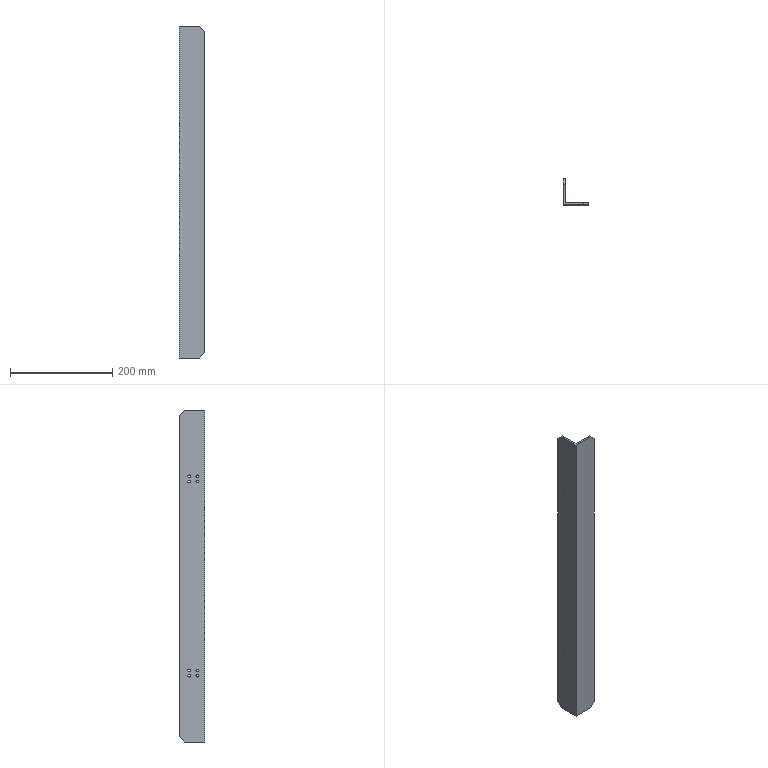Part | SolidWorks | features Chamfer 1, Extrusion 1, HoleWzd 1 | 1 solid | 44 faces | box 50 x 50 x 650 mm | volume 247288 mm3 | cylinder 16 | cone 16 | plane 12 | commonest cylinder face diameters 5.5 x16
STEP:
#1=CARTESIAN_POINT('',(0.,30.5,197.75));
#2=VERTEX_POINT('',#1);
#3=CARTESIAN_POINT('',(0.,30.5,192.25));
#4=VERTEX_POINT('',#3);
#5=CARTESIAN_POINT('',(0.,30.5,195.));
#6=DIRECTION('',(1.,0.,0.));
#7=DIRECTION('',(0.,0.,-1.));
#8=AXIS2_PLACEMENT_3D('',#5,#6,#7);
#9=CIRCLE('',#8,2.75);
#10=EDGE_CURVE('',#2,#4,#9,.T.);
#11=ORIENTED_EDGE('',*,*,#10,.F.);
#12=CARTESIAN_POINT('',(1.15,30.5,197.75));
#13=VERTEX_POINT('',#12);
#14=CARTESIAN_POINT('',(4.,30.5,197.75));
#15=DIRECTION('',(1.,0.,0.));
#16=VECTOR('',#15,1000.);
#17=LINE('',#14,#16);
#18=EDGE_CURVE('',#2,#13,#17,.T.);
#19=ORIENTED_EDGE('',*,*,#18,.T.);
#20=CARTESIAN_POINT('',(1.15,30.5,192.25));
#21=VERTEX_POINT('',#20);
#22=CARTESIAN_POINT('',(1.15,30.5,195.));
#23=DIRECTION('',(1.,0.,0.));
#24=DIRECTION('',(0.,0.,-1.));
#25=AXIS2_PLACEMENT_3D('',#22,#23,#24);
#26=CIRCLE('',#25,2.75);
#27=EDGE_CURVE('',#13,#21,#26,.T.);
#28=ORIENTED_EDGE('',*,*,#27,.T.);
#29=CARTESIAN_POINT('',(4.,30.5,192.25));
#30=DIRECTION('',(1.,0.,0.));
#31=VECTOR('',#30,1000.);
#32=LINE('',#29,#31);
#33=EDGE_CURVE('',#4,#21,#32,.T.);
#34=ORIENTED_EDGE('',*,*,#33,.F.);
#35=EDGE_LOOP('',(#11,#19,#28,#34));
#36=FACE_OUTER_BOUND('',#35,.T.);
#37=CARTESIAN_POINT('',(4.,30.5,195.));
#38=DIRECTION('',(1.,0.,0.));
#39=DIRECTION('',(0.,0.,-1.));
#40=AXIS2_PLACEMENT_3D('',#37,#38,#39);
#41=CYLINDRICAL_SURFACE('',#40,2.75);
#42=ADVANCED_FACE('',(#36),#41,.F.);
#43=ORIENTED_EDGE('',*,*,#27,.F.);
#44=CARTESIAN_POINT('',(4.,30.5,200.6));
#45=VERTEX_POINT('',#44);
#46=CARTESIAN_POINT('',(4.,30.5,200.6));
#47=DIRECTION('',(0.7071,0.,0.7071));
#48=VECTOR('',#47,1000.);
#49=LINE('',#46,#48);
#50=EDGE_CURVE('',#13,#45,#49,.T.);
#51=ORIENTED_EDGE('',*,*,#50,.T.);
#52=CARTESIAN_POINT('',(4.,27.978,190.));
#53=VERTEX_POINT('',#52);
#54=CARTESIAN_POINT('',(4.,30.5,195.));
#55=DIRECTION('',(1.,0.,0.));
#56=DIRECTION('',(0.,0.,-1.));
#57=AXIS2_PLACEMENT_3D('',#54,#55,#56);
#58=CIRCLE('',#57,5.6);
#59=EDGE_CURVE('',#45,#53,#58,.T.);
#60=ORIENTED_EDGE('',*,*,#59,.T.);
#61=CARTESIAN_POINT('',(3.4,30.5,190.));
#62=VERTEX_POINT('',#61);
#63=CARTESIAN_POINT('',(3.4,30.5,190.));
#64=CARTESIAN_POINT('',(3.4,30.063,190.));
#65=CARTESIAN_POINT('',(3.458,29.635,190.));
#66=CARTESIAN_POINT('',(3.668,28.793,190.));
#67=CARTESIAN_POINT('',(3.82,28.378,190.));
#68=CARTESIAN_POINT('',(4.,27.978,190.));
#69=B_SPLINE_CURVE_WITH_KNOTS('',3,(#63,#64,#65,#66,#67,#68),.UNSPECIFIED.,.F.,.F.,(4,2,4),(0.002595,0.003891,0.005187),.UNSPECIFIED.);
#70=EDGE_CURVE('',#62,#53,#69,.T.);
#71=ORIENTED_EDGE('',*,*,#70,.F.);
#72=CARTESIAN_POINT('',(4.,30.5,189.4));
#73=DIRECTION('',(0.7071,0.,-0.7071));
#74=VECTOR('',#73,1000.);
#75=LINE('',#72,#74);
#76=EDGE_CURVE('',#21,#62,#75,.T.);
#77=ORIENTED_EDGE('',*,*,#76,.F.);
#78=EDGE_LOOP('',(#43,#51,#60,#71,#77));
#79=FACE_OUTER_BOUND('',#78,.T.);
#80=CARTESIAN_POINT('',(4.,30.5,195.));
#81=DIRECTION('',(1.,0.,0.));
#82=DIRECTION('',(0.,0.,-1.));
#83=AXIS2_PLACEMENT_3D('',#80,#81,#82);
#84=CONICAL_SURFACE('',#83,5.6,0.7854);
#85=ADVANCED_FACE('',(#79),#84,.F.);
#86=CARTESIAN_POINT('',(0.,30.5,-182.25));
#87=VERTEX_POINT('',#86);
#88=CARTESIAN_POINT('',(0.,30.5,-187.75));
#89=VERTEX_POINT('',#88);
#90=CARTESIAN_POINT('',(0.,30.5,-185.));
#91=DIRECTION('',(1.,0.,0.));
#92=DIRECTION('',(0.,0.,-1.));
#93=AXIS2_PLACEMENT_3D('',#90,#91,#92);
#94=CIRCLE('',#93,2.75);
#95=EDGE_CURVE('',#87,#89,#94,.T.);
#96=ORIENTED_EDGE('',*,*,#95,.F.);
#97=CARTESIAN_POINT('',(1.15,30.5,-182.25));
#98=VERTEX_POINT('',#97);
#99=CARTESIAN_POINT('',(4.,30.5,-182.25));
#100=DIRECTION('',(1.,0.,0.));
#101=VECTOR('',#100,1000.);
#102=LINE('',#99,#101);
#103=EDGE_CURVE('',#87,#98,#102,.T.);
#104=ORIENTED_EDGE('',*,*,#103,.T.);
#105=CARTESIAN_POINT('',(1.15,30.5,-187.75));
#106=VERTEX_POINT('',#105);
#107=CARTESIAN_POINT('',(1.15,30.5,-185.));
#108=DIRECTION('',(1.,0.,0.));
#109=DIRECTION('',(0.,0.,-1.));
#110=AXIS2_PLACEMENT_3D('',#107,#108,#109);
#111=CIRCLE('',#110,2.75);
#112=EDGE_CURVE('',#98,#106,#111,.T.);
#113=ORIENTED_EDGE('',*,*,#112,.T.);
#114=CARTESIAN_POINT('',(4.,30.5,-187.75));
#115=DIRECTION('',(1.,0.,0.));
#116=VECTOR('',#115,1000.);
#117=LINE('',#114,#116);
#118=EDGE_CURVE('',#89,#106,#117,.T.);
#119=ORIENTED_EDGE('',*,*,#118,.F.);
#120=EDGE_LOOP('',(#96,#104,#113,#119));
#121=FACE_OUTER_BOUND('',#120,.T.);
#122=CARTESIAN_POINT('',(4.,30.5,-185.));
#123=DIRECTION('',(1.,0.,0.));
#124=DIRECTION('',(0.,0.,-1.));
#125=AXIS2_PLACEMENT_3D('',#122,#123,#124);
#126=CYLINDRICAL_SURFACE('',#125,2.75);
#127=ADVANCED_FACE('',(#121),#126,.F.);
#128=ORIENTED_EDGE('',*,*,#112,.F.);
#129=CARTESIAN_POINT('',(4.,30.5,-179.4));
#130=VERTEX_POINT('',#129);
#131=CARTESIAN_POINT('',(4.,30.5,-179.4));
#132=DIRECTION('',(0.7071,0.,0.7071));
#133=VECTOR('',#132,1000.);
#134=LINE('',#131,#133);
#135=EDGE_CURVE('',#98,#130,#134,.T.);
#136=ORIENTED_EDGE('',*,*,#135,.T.);
#137=CARTESIAN_POINT('',(4.,27.978,-190.));
#138=VERTEX_POINT('',#137);
#139=CARTESIAN_POINT('',(4.,30.5,-185.));
#140=DIRECTION('',(1.,0.,0.));
#141=DIRECTION('',(0.,0.,-1.));
#142=AXIS2_PLACEMENT_3D('',#139,#140,#141);
#143=CIRCLE('',#142,5.6);
#144=EDGE_CURVE('',#130,#138,#143,.T.);
#145=ORIENTED_EDGE('',*,*,#144,.T.);
#146=CARTESIAN_POINT('',(3.4,30.5,-190.));
#147=VERTEX_POINT('',#146);
#148=CARTESIAN_POINT('',(3.4,30.5,-190.));
#149=CARTESIAN_POINT('',(3.4,30.063,-190.));
#150=CARTESIAN_POINT('',(3.458,29.635,-190.));
#151=CARTESIAN_POINT('',(3.668,28.793,-190.));
#152=CARTESIAN_POINT('',(3.82,28.378,-190.));
#153=CARTESIAN_POINT('',(4.,27.978,-190.));
#154=B_SPLINE_CURVE_WITH_KNOTS('',3,(#148,#149,#150,#151,#152,#153),.UNSPECIFIED.,.F.,.F.,(4,2,4),(0.002595,0.003891,0.005187),.UNSPECIFIED.);
#155=EDGE_CURVE('',#147,#138,#154,.T.);
#156=ORIENTED_EDGE('',*,*,#155,.F.);
#157=CARTESIAN_POINT('',(4.,30.5,-190.6));
#158=DIRECTION('',(0.7071,0.,-0.7071));
#159=VECTOR('',#158,1000.);
#160=LINE('',#157,#159);
#161=EDGE_CURVE('',#106,#147,#160,.T.);
#162=ORIENTED_EDGE('',*,*,#161,.F.);
#163=EDGE_LOOP('',(#128,#136,#145,#156,#162));
#164=FACE_OUTER_BOUND('',#163,.T.);
#165=CARTESIAN_POINT('',(4.,30.5,-185.));
#166=DIRECTION('',(1.,0.,0.));
#167=DIRECTION('',(0.,0.,-1.));
#168=AXIS2_PLACEMENT_3D('',#165,#166,#167);
#169=CONICAL_SURFACE('',#168,5.6,0.7854);
#170=ADVANCED_FACE('',(#164),#169,.F.);
#171=CARTESIAN_POINT('',(1.15,30.5,187.75));
#172=VERTEX_POINT('',#171);
#173=CARTESIAN_POINT('',(1.15,30.5,182.25));
#174=VERTEX_POINT('',#173);
#175=CARTESIAN_POINT('',(1.15,30.5,185.));
#176=DIRECTION('',(1.,0.,0.));
#177=DIRECTION('',(0.,0.,-1.));
#178=AXIS2_PLACEMENT_3D('',#175,#176,#177);
#179=CIRCLE('',#178,2.75);
#180=EDGE_CURVE('',#172,#174,#179,.T.);
#181=ORIENTED_EDGE('',*,*,#180,.F.);
#182=CARTESIAN_POINT('',(4.,30.5,190.6));
#183=DIRECTION('',(0.7071,0.,0.7071));
#184=VECTOR('',#183,1000.);
#185=LINE('',#182,#184);
#186=EDGE_CURVE('',#172,#62,#185,.T.);
#187=ORIENTED_EDGE('',*,*,#186,.T.);
#188=ORIENTED_EDGE('',*,*,#70,.T.);
#189=CARTESIAN_POINT('',(4.,30.5,179.4));
#190=VERTEX_POINT('',#189);
#191=CARTESIAN_POINT('',(4.,30.5,185.));
#192=DIRECTION('',(1.,0.,0.));
#193=DIRECTION('',(0.,0.,-1.));
#194=AXIS2_PLACEMENT_3D('',#191,#192,#193);
#195=CIRCLE('',#194,5.6);
#196=EDGE_CURVE('',#53,#190,#195,.T.);
#197=ORIENTED_EDGE('',*,*,#196,.T.);
#198=CARTESIAN_POINT('',(4.,30.5,179.4));
#199=DIRECTION('',(0.7071,0.,-0.7071));
#200=VECTOR('',#199,1000.);
#201=LINE('',#198,#200);
#202=EDGE_CURVE('',#174,#190,#201,.T.);
#203=ORIENTED_EDGE('',*,*,#202,.F.);
#204=EDGE_LOOP('',(#181,#187,#188,#197,#203));
#205=FACE_OUTER_BOUND('',#204,.T.);
#206=CARTESIAN_POINT('',(4.,30.5,185.));
#207=DIRECTION('',(1.,0.,0.));
#208=DIRECTION('',(0.,0.,-1.));
#209=AXIS2_PLACEMENT_3D('',#206,#207,#208);
#210=CONICAL_SURFACE('',#209,5.6,0.7854);
#211=ADVANCED_FACE('',(#205),#210,.F.);
#212=CARTESIAN_POINT('',(0.,30.5,187.75));
#213=VERTEX_POINT('',#212);
#214=CARTESIAN_POINT('',(0.,30.5,182.25));
#215=VERTEX_POINT('',#214);
#216=CARTESIAN_POINT('',(0.,30.5,185.));
#217=DIRECTION('',(1.,0.,0.));
#218=DIRECTION('',(0.,0.,-1.));
#219=AXIS2_PLACEMENT_3D('',#216,#217,#218);
#220=CIRCLE('',#219,2.75);
#221=EDGE_CURVE('',#213,#215,#220,.T.);
#222=ORIENTED_EDGE('',*,*,#221,.F.);
#223=CARTESIAN_POINT('',(4.,30.5,187.75));
#224=DIRECTION('',(1.,0.,0.));
#225=VECTOR('',#224,1000.);
#226=LINE('',#223,#225);
#227=EDGE_CURVE('',#213,#172,#226,.T.);
#228=ORIENTED_EDGE('',*,*,#227,.T.);
#229=ORIENTED_EDGE('',*,*,#180,.T.);
#230=CARTESIAN_POINT('',(4.,30.5,182.25));
#231=DIRECTION('',(1.,0.,0.));
#232=VECTOR('',#231,1000.);
#233=LINE('',#230,#232);
#234=EDGE_CURVE('',#215,#174,#233,.T.);
#235=ORIENTED_EDGE('',*,*,#234,.F.);
#236=EDGE_LOOP('',(#222,#228,#229,#235));
#237=FACE_OUTER_BOUND('',#236,.T.);
#238=CARTESIAN_POINT('',(4.,30.5,185.));
#239=DIRECTION('',(1.,0.,0.));
#240=DIRECTION('',(0.,0.,-1.));
#241=AXIS2_PLACEMENT_3D('',#238,#239,#240);
#242=CYLINDRICAL_SURFACE('',#241,2.75);
#243=ADVANCED_FACE('',(#237),#242,.F.);
#244=CARTESIAN_POINT('',(1.15,30.5,-192.25));
#245=VERTEX_POINT('',#244);
#246=CARTESIAN_POINT('',(1.15,30.5,-197.75));
#247=VERTEX_POINT('',#246);
#248=CARTESIAN_POINT('',(1.15,30.5,-195.));
#249=DIRECTION('',(1.,0.,0.));
#250=DIRECTION('',(0.,0.,-1.));
#251=AXIS2_PLACEMENT_3D('',#248,#249,#250);
#252=CIRCLE('',#251,2.75);
#253=EDGE_CURVE('',#245,#247,#252,.T.);
#254=ORIENTED_EDGE('',*,*,#253,.F.);
#255=CARTESIAN_POINT('',(4.,30.5,-189.4));
#256=DIRECTION('',(0.7071,0.,0.7071));
#257=VECTOR('',#256,1000.);
#258=LINE('',#255,#257);
#259=EDGE_CURVE('',#245,#147,#258,.T.);
#260=ORIENTED_EDGE('',*,*,#259,.T.);
#261=ORIENTED_EDGE('',*,*,#155,.T.);
#262=CARTESIAN_POINT('',(4.,30.5,-200.6));
#263=VERTEX_POINT('',#262);
#264=CARTESIAN_POINT('',(4.,30.5,-195.));
#265=DIRECTION('',(1.,0.,0.));
#266=DIRECTION('',(0.,0.,-1.));
#267=AXIS2_PLACEMENT_3D('',#264,#265,#266);
#268=CIRCLE('',#267,5.6);
#269=EDGE_CURVE('',#138,#263,#268,.T.);
#270=ORIENTED_EDGE('',*,*,#269,.T.);
#271=CARTESIAN_POINT('',(4.,30.5,-200.6));
#272=DIRECTION('',(0.7071,0.,-0.7071));
#273=VECTOR('',#272,1000.);
#274=LINE('',#271,#273);
#275=EDGE_CURVE('',#247,#263,#274,.T.);
#276=ORIENTED_EDGE('',*,*,#275,.F.);
#277=EDGE_LOOP('',(#254,#260,#261,#270,#276));
#278=FACE_OUTER_BOUND('',#277,.T.);
#279=CARTESIAN_POINT('',(4.,30.5,-195.));
#280=DIRECTION('',(1.,0.,0.));
#281=DIRECTION('',(0.,0.,-1.));
#282=AXIS2_PLACEMENT_3D('',#279,#280,#281);
#283=CONICAL_SURFACE('',#282,5.6,0.7854);
#284=ADVANCED_FACE('',(#278),#283,.F.);
#285=CARTESIAN_POINT('',(0.,30.5,-192.25));
#286=VERTEX_POINT('',#285);
#287=CARTESIAN_POINT('',(0.,30.5,-197.75));
#288=VERTEX_POINT('',#287);
#289=CARTESIAN_POINT('',(0.,30.5,-195.));
#290=DIRECTION('',(1.,0.,0.));
#291=DIRECTION('',(0.,0.,-1.));
#292=AXIS2_PLACEMENT_3D('',#289,#290,#291);
#293=CIRCLE('',#292,2.75);
#294=EDGE_CURVE('',#286,#288,#293,.T.);
#295=ORIENTED_EDGE('',*,*,#294,.F.);
#296=CARTESIAN_POINT('',(4.,30.5,-192.25));
#297=DIRECTION('',(1.,0.,0.));
#298=VECTOR('',#297,1000.);
#299=LINE('',#296,#298);
#300=EDGE_CURVE('',#286,#245,#299,.T.);
#301=ORIENTED_EDGE('',*,*,#300,.T.);
#302=ORIENTED_EDGE('',*,*,#253,.T.);
#303=CARTESIAN_POINT('',(4.,30.5,-197.75));
#304=DIRECTION('',(1.,0.,0.));
#305=VECTOR('',#304,1000.);
#306=LINE('',#303,#305);
#307=EDGE_CURVE('',#288,#247,#306,.T.);
#308=ORIENTED_EDGE('',*,*,#307,.F.);
#309=EDGE_LOOP('',(#295,#301,#302,#308));
#310=FACE_OUTER_BOUND('',#309,.T.);
#311=CARTESIAN_POINT('',(4.,30.5,-195.));
#312=DIRECTION('',(1.,0.,0.));
#313=DIRECTION('',(0.,0.,-1.));
#314=AXIS2_PLACEMENT_3D('',#311,#312,#313);
#315=CYLINDRICAL_SURFACE('',#314,2.75);
#316=ADVANCED_FACE('',(#310),#315,.F.);
#317=CARTESIAN_POINT('',(0.,14.5,197.75));
#318=VERTEX_POINT('',#317);
#319=CARTESIAN_POINT('',(0.,14.5,192.25));
#320=VERTEX_POINT('',#319);
#321=CARTESIAN_POINT('',(0.,14.5,195.));
#322=DIRECTION('',(1.,0.,0.));
#323=DIRECTION('',(0.,0.,-1.));
#324=AXIS2_PLACEMENT_3D('',#321,#322,#323);
#325=CIRCLE('',#324,2.75);
#326=EDGE_CURVE('',#318,#320,#325,.T.);
#327=ORIENTED_EDGE('',*,*,#326,.F.);
#328=CARTESIAN_POINT('',(1.15,14.5,197.75));
#329=VERTEX_POINT('',#328);
#330=CARTESIAN_POINT('',(4.,14.5,197.75));
#331=DIRECTION('',(1.,0.,0.));
#332=VECTOR('',#331,1000.);
#333=LINE('',#330,#332);
#334=EDGE_CURVE('',#318,#329,#333,.T.);
#335=ORIENTED_EDGE('',*,*,#334,.T.);
#336=CARTESIAN_POINT('',(1.15,14.5,192.25));
#337=VERTEX_POINT('',#336);
#338=CARTESIAN_POINT('',(1.15,14.5,195.));
#339=DIRECTION('',(1.,0.,0.));
#340=DIRECTION('',(0.,0.,-1.));
#341=AXIS2_PLACEMENT_3D('',#338,#339,#340);
#342=CIRCLE('',#341,2.75);
#343=EDGE_CURVE('',#329,#337,#342,.T.);
#344=ORIENTED_EDGE('',*,*,#343,.T.);
#345=CARTESIAN_POINT('',(4.,14.5,192.25));
#346=DIRECTION('',(1.,0.,0.));
#347=VECTOR('',#346,1000.);
#348=LINE('',#345,#347);
#349=EDGE_CURVE('',#320,#337,#348,.T.);
#350=ORIENTED_EDGE('',*,*,#349,.F.);
#351=EDGE_LOOP('',(#327,#335,#344,#350));
#352=FACE_OUTER_BOUND('',#351,.T.);
#353=CARTESIAN_POINT('',(4.,14.5,195.));
#354=DIRECTION('',(1.,0.,0.));
#355=DIRECTION('',(0.,0.,-1.));
#356=AXIS2_PLACEMENT_3D('',#353,#354,#355);
#357=CYLINDRICAL_SURFACE('',#356,2.75);
#358=ADVANCED_FACE('',(#352),#357,.F.);
#359=ORIENTED_EDGE('',*,*,#343,.F.);
#360=CARTESIAN_POINT('',(4.,14.5,200.6));
#361=VERTEX_POINT('',#360);
#362=CARTESIAN_POINT('',(4.,14.5,200.6));
#363=DIRECTION('',(0.7071,0.,0.7071));
#364=VECTOR('',#363,1000.);
#365=LINE('',#362,#364);
#366=EDGE_CURVE('',#329,#361,#365,.T.);
#367=ORIENTED_EDGE('',*,*,#366,.T.);
#368=CARTESIAN_POINT('',(4.,11.978,190.));
#369=VERTEX_POINT('',#368);
#370=CARTESIAN_POINT('',(4.,14.5,195.));
#371=DIRECTION('',(1.,0.,0.));
#372=DIRECTION('',(0.,0.,-1.));
#373=AXIS2_PLACEMENT_3D('',#370,#371,#372);
#374=CIRCLE('',#373,5.6);
#375=EDGE_CURVE('',#361,#369,#374,.T.);
#376=ORIENTED_EDGE('',*,*,#375,.T.);
#377=CARTESIAN_POINT('',(3.4,14.5,190.));
#378=VERTEX_POINT('',#377);
#379=CARTESIAN_POINT('',(3.4,14.5,190.));
#380=CARTESIAN_POINT('',(3.4,14.063,190.));
#381=CARTESIAN_POINT('',(3.458,13.635,190.));
#382=CARTESIAN_POINT('',(3.668,12.793,190.));
#383=CARTESIAN_POINT('',(3.82,12.378,190.));
#384=CARTESIAN_POINT('',(4.,11.978,190.));
#385=B_SPLINE_CURVE_WITH_KNOTS('',3,(#379,#380,#381,#382,#383,#384),.UNSPECIFIED.,.F.,.F.,(4,2,4),(0.002595,0.003891,0.005187),.UNSPECIFIED.);
#386=EDGE_CURVE('',#378,#369,#385,.T.);
#387=ORIENTED_EDGE('',*,*,#386,.F.);
#388=CARTESIAN_POINT('',(4.,14.5,189.4));
#389=DIRECTION('',(0.7071,0.,-0.7071));
#390=VECTOR('',#389,1000.);
#391=LINE('',#388,#390);
#392=EDGE_CURVE('',#337,#378,#391,.T.);
#393=ORIENTED_EDGE('',*,*,#392,.F.);
#394=EDGE_LOOP('',(#359,#367,#376,#387,#393));
#395=FACE_OUTER_BOUND('',#394,.T.);
#396=CARTESIAN_POINT('',(4.,14.5,195.));
#397=DIRECTION('',(1.,0.,0.));
#398=DIRECTION('',(0.,0.,-1.));
#399=AXIS2_PLACEMENT_3D('',#396,#397,#398);
#400=CONICAL_SURFACE('',#399,5.6,0.7854);
#401=ADVANCED_FACE('',(#395),#400,.F.);
#402=CARTESIAN_POINT('',(0.,14.5,-182.25));
#403=VERTEX_POINT('',#402);
#404=CARTESIAN_POINT('',(0.,14.5,-187.75));
#405=VERTEX_POINT('',#404);
#406=CARTESIAN_POINT('',(0.,14.5,-185.));
#407=DIRECTION('',(1.,0.,0.));
#408=DIRECTION('',(0.,0.,-1.));
#409=AXIS2_PLACEMENT_3D('',#406,#407,#408);
#410=CIRCLE('',#409,2.75);
#411=EDGE_CURVE('',#403,#405,#410,.T.);
#412=ORIENTED_EDGE('',*,*,#411,.F.);
#413=CARTESIAN_POINT('',(1.15,14.5,-182.25));
#414=VERTEX_POINT('',#413);
#415=CARTESIAN_POINT('',(4.,14.5,-182.25));
#416=DIRECTION('',(1.,0.,0.));
#417=VECTOR('',#416,1000.);
#418=LINE('',#415,#417);
#419=EDGE_CURVE('',#403,#414,#418,.T.);
#420=ORIENTED_EDGE('',*,*,#419,.T.);
#421=CARTESIAN_POINT('',(1.15,14.5,-187.75));
#422=VERTEX_POINT('',#421);
#423=CARTESIAN_POINT('',(1.15,14.5,-185.));
#424=DIRECTION('',(1.,0.,0.));
#425=DIRECTION('',(0.,0.,-1.));
#426=AXIS2_PLACEMENT_3D('',#423,#424,#425);
#427=CIRCLE('',#426,2.75);
#428=EDGE_CURVE('',#414,#422,#427,.T.);
#429=ORIENTED_EDGE('',*,*,#428,.T.);
#430=CARTESIAN_POINT('',(4.,14.5,-187.75));
#431=DIRECTION('',(1.,0.,0.));
#432=VECTOR('',#431,1000.);
#433=LINE('',#430,#432);
#434=EDGE_CURVE('',#405,#422,#433,.T.);
#435=ORIENTED_EDGE('',*,*,#434,.F.);
#436=EDGE_LOOP('',(#412,#420,#429,#435));
#437=FACE_OUTER_BOUND('',#436,.T.);
#438=CARTESIAN_POINT('',(4.,14.5,-185.));
#439=DIRECTION('',(1.,0.,0.));
#440=DIRECTION('',(0.,0.,-1.));
#441=AXIS2_PLACEMENT_3D('',#438,#439,#440);
#442=CYLINDRICAL_SURFACE('',#441,2.75);
#443=ADVANCED_FACE('',(#437),#442,.F.);
#444=ORIENTED_EDGE('',*,*,#428,.F.);
#445=CARTESIAN_POINT('',(4.,14.5,-179.4));
#446=VERTEX_POINT('',#445);
#447=CARTESIAN_POINT('',(4.,14.5,-179.4));
#448=DIRECTION('',(0.7071,0.,0.7071));
#449=VECTOR('',#448,1000.);
#450=LINE('',#447,#449);
#451=EDGE_CURVE('',#414,#446,#450,.T.);
#452=ORIENTED_EDGE('',*,*,#451,.T.);
#453=CARTESIAN_POINT('',(4.,11.978,-190.));
#454=VERTEX_POINT('',#453);
#455=CARTESIAN_POINT('',(4.,14.5,-185.));
#456=DIRECTION('',(1.,0.,0.));
#457=DIRECTION('',(0.,0.,-1.));
#458=AXIS2_PLACEMENT_3D('',#455,#456,#457);
#459=CIRCLE('',#458,5.6);
#460=EDGE_CURVE('',#446,#454,#459,.T.);
#461=ORIENTED_EDGE('',*,*,#460,.T.);
#462=CARTESIAN_POINT('',(3.4,14.5,-190.));
#463=VERTEX_POINT('',#462);
#464=CARTESIAN_POINT('',(3.4,14.5,-190.));
#465=CARTESIAN_POINT('',(3.4,14.063,-190.));
#466=CARTESIAN_POINT('',(3.458,13.635,-190.));
#467=CARTESIAN_POINT('',(3.668,12.793,-190.));
#468=CARTESIAN_POINT('',(3.82,12.378,-190.));
#469=CARTESIAN_POINT('',(4.,11.978,-190.));
#470=B_SPLINE_CURVE_WITH_KNOTS('',3,(#464,#465,#466,#467,#468,#469),.UNSPECIFIED.,.F.,.F.,(4,2,4),(0.002595,0.003891,0.005187),.UNSPECIFIED.);
#471=EDGE_CURVE('',#463,#454,#470,.T.);
#472=ORIENTED_EDGE('',*,*,#471,.F.);
#473=CARTESIAN_POINT('',(4.,14.5,-190.6));
#474=DIRECTION('',(0.7071,0.,-0.7071));
#475=VECTOR('',#474,1000.);
#476=LINE('',#473,#475);
#477=EDGE_CURVE('',#422,#463,#476,.T.);
#478=ORIENTED_EDGE('',*,*,#477,.F.);
#479=EDGE_LOOP('',(#444,#452,#461,#472,#478));
#480=FACE_OUTER_BOUND('',#479,.T.);
#481=CARTESIAN_POINT('',(4.,14.5,-185.));
#482=DIRECTION('',(1.,0.,0.));
#483=DIRECTION('',(0.,0.,-1.));
#484=AXIS2_PLACEMENT_3D('',#481,#482,#483);
#485=CONICAL_SURFACE('',#484,5.6,0.7854);
#486=ADVANCED_FACE('',(#480),#485,.F.);
#487=CARTESIAN_POINT('',(1.15,14.5,187.75));
#488=VERTEX_POINT('',#487);
#489=CARTESIAN_POINT('',(1.15,14.5,182.25));
#490=VERTEX_POINT('',#489);
#491=CARTESIAN_POINT('',(1.15,14.5,185.));
#492=DIRECTION('',(1.,0.,0.));
#493=DIRECTION('',(0.,0.,-1.));
#494=AXIS2_PLACEMENT_3D('',#491,#492,#493);
#495=CIRCLE('',#494,2.75);
#496=EDGE_CURVE('',#488,#490,#495,.T.);
#497=ORIENTED_EDGE('',*,*,#496,.F.);
#498=CARTESIAN_POINT('',(4.,14.5,190.6));
#499=DIRECTION('',(0.7071,0.,0.7071));
#500=VECTOR('',#499,1000.);
#501=LINE('',#498,#500);
#502=EDGE_CURVE('',#488,#378,#501,.T.);
#503=ORIENTED_EDGE('',*,*,#502,.T.);
#504=ORIENTED_EDGE('',*,*,#386,.T.);
#505=CARTESIAN_POINT('',(4.,14.5,179.4));
#506=VERTEX_POINT('',#505);
#507=CARTESIAN_POINT('',(4.,14.5,185.));
#508=DIRECTION('',(1.,0.,0.));
#509=DIRECTION('',(0.,0.,-1.));
#510=AXIS2_PLACEMENT_3D('',#507,#508,#509);
#511=CIRCLE('',#510,5.6);
#512=EDGE_CURVE('',#369,#506,#511,.T.);
#513=ORIENTED_EDGE('',*,*,#512,.T.);
#514=CARTESIAN_POINT('',(4.,14.5,179.4));
#515=DIRECTION('',(0.7071,0.,-0.7071));
#516=VECTOR('',#515,1000.);
#517=LINE('',#514,#516);
#518=EDGE_CURVE('',#490,#506,#517,.T.);
#519=ORIENTED_EDGE('',*,*,#518,.F.);
#520=EDGE_LOOP('',(#497,#503,#504,#513,#519));
#521=FACE_OUTER_BOUND('',#520,.T.);
#522=CARTESIAN_POINT('',(4.,14.5,185.));
#523=DIRECTION('',(1.,0.,0.));
#524=DIRECTION('',(0.,0.,-1.));
#525=AXIS2_PLACEMENT_3D('',#522,#523,#524);
#526=CONICAL_SURFACE('',#525,5.6,0.7854);
#527=ADVANCED_FACE('',(#521),#526,.F.);
#528=CARTESIAN_POINT('',(0.,14.5,187.75));
#529=VERTEX_POINT('',#528);
#530=CARTESIAN_POINT('',(0.,14.5,182.25));
#531=VERTEX_POINT('',#530);
#532=CARTESIAN_POINT('',(0.,14.5,185.));
#533=DIRECTION('',(1.,0.,0.));
#534=DIRECTION('',(0.,0.,-1.));
#535=AXIS2_PLACEMENT_3D('',#532,#533,#534);
#536=CIRCLE('',#535,2.75);
#537=EDGE_CURVE('',#529,#531,#536,.T.);
#538=ORIENTED_EDGE('',*,*,#537,.F.);
#539=CARTESIAN_POINT('',(4.,14.5,187.75));
#540=DIRECTION('',(1.,0.,0.));
#541=VECTOR('',#540,1000.);
#542=LINE('',#539,#541);
#543=EDGE_CURVE('',#529,#488,#542,.T.);
#544=ORIENTED_EDGE('',*,*,#543,.T.);
#545=ORIENTED_EDGE('',*,*,#496,.T.);
#546=CARTESIAN_POINT('',(4.,14.5,182.25));
#547=DIRECTION('',(1.,0.,0.));
#548=VECTOR('',#547,1000.);
#549=LINE('',#546,#548);
#550=EDGE_CURVE('',#531,#490,#549,.T.);
#551=ORIENTED_EDGE('',*,*,#550,.F.);
#552=EDGE_LOOP('',(#538,#544,#545,#551));
#553=FACE_OUTER_BOUND('',#552,.T.);
#554=CARTESIAN_POINT('',(4.,14.5,185.));
#555=DIRECTION('',(1.,0.,0.));
#556=DIRECTION('',(0.,0.,-1.));
#557=AXIS2_PLACEMENT_3D('',#554,#555,#556);
#558=CYLINDRICAL_SURFACE('',#557,2.75);
#559=ADVANCED_FACE('',(#553),#558,.F.);
#560=CARTESIAN_POINT('',(1.15,14.5,-192.25));
#561=VERTEX_POINT('',#560);
#562=CARTESIAN_POINT('',(1.15,14.5,-197.75));
#563=VERTEX_POINT('',#562);
#564=CARTESIAN_POINT('',(1.15,14.5,-195.));
#565=DIRECTION('',(1.,0.,0.));
#566=DIRECTION('',(0.,0.,-1.));
#567=AXIS2_PLACEMENT_3D('',#564,#565,#566);
#568=CIRCLE('',#567,2.75);
#569=EDGE_CURVE('',#561,#563,#568,.T.);
#570=ORIENTED_EDGE('',*,*,#569,.F.);
#571=CARTESIAN_POINT('',(4.,14.5,-189.4));
#572=DIRECTION('',(0.7071,0.,0.7071));
#573=VECTOR('',#572,1000.);
#574=LINE('',#571,#573);
#575=EDGE_CURVE('',#561,#463,#574,.T.);
#576=ORIENTED_EDGE('',*,*,#575,.T.);
#577=ORIENTED_EDGE('',*,*,#471,.T.);
#578=CARTESIAN_POINT('',(4.,14.5,-200.6));
#579=VERTEX_POINT('',#578);
#580=CARTESIAN_POINT('',(4.,14.5,-195.));
#581=DIRECTION('',(1.,0.,0.));
#582=DIRECTION('',(0.,0.,-1.));
#583=AXIS2_PLACEMENT_3D('',#580,#581,#582);
#584=CIRCLE('',#583,5.6);
#585=EDGE_CURVE('',#454,#579,#584,.T.);
#586=ORIENTED_EDGE('',*,*,#585,.T.);
#587=CARTESIAN_POINT('',(4.,14.5,-200.6));
#588=DIRECTION('',(0.7071,0.,-0.7071));
#589=VECTOR('',#588,1000.);
#590=LINE('',#587,#589);
#591=EDGE_CURVE('',#563,#579,#590,.T.);
#592=ORIENTED_EDGE('',*,*,#591,.F.);
#593=EDGE_LOOP('',(#570,#576,#577,#586,#592));
#594=FACE_OUTER_BOUND('',#593,.T.);
#595=CARTESIAN_POINT('',(4.,14.5,-195.));
#596=DIRECTION('',(1.,0.,0.));
#597=DIRECTION('',(0.,0.,-1.));
#598=AXIS2_PLACEMENT_3D('',#595,#596,#597);
#599=CONICAL_SURFACE('',#598,5.6,0.7854);
#600=ADVANCED_FACE('',(#594),#599,.F.);
#601=CARTESIAN_POINT('',(0.,14.5,-192.25));
#602=VERTEX_POINT('',#601);
#603=CARTESIAN_POINT('',(0.,14.5,-197.75));
#604=VERTEX_POINT('',#603);
#605=CARTESIAN_POINT('',(0.,14.5,-195.));
#606=DIRECTION('',(1.,0.,0.));
#607=DIRECTION('',(0.,0.,-1.));
#608=AXIS2_PLACEMENT_3D('',#605,#606,#607);
#609=CIRCLE('',#608,2.75);
#610=EDGE_CURVE('',#602,#604,#609,.T.);
#611=ORIENTED_EDGE('',*,*,#610,.F.);
#612=CARTESIAN_POINT('',(4.,14.5,-192.25));
#613=DIRECTION('',(1.,0.,0.));
#614=VECTOR('',#613,1000.);
#615=LINE('',#612,#614);
#616=EDGE_CURVE('',#602,#561,#615,.T.);
#617=ORIENTED_EDGE('',*,*,#616,.T.);
#618=ORIENTED_EDGE('',*,*,#569,.T.);
#619=CARTESIAN_POINT('',(4.,14.5,-197.75));
#620=DIRECTION('',(1.,0.,0.));
#621=VECTOR('',#620,1000.);
#622=LINE('',#619,#621);
#623=EDGE_CURVE('',#604,#563,#622,.T.);
#624=ORIENTED_EDGE('',*,*,#623,.F.);
#625=EDGE_LOOP('',(#611,#617,#618,#624));
#626=FACE_OUTER_BOUND('',#625,.T.);
#627=CARTESIAN_POINT('',(4.,14.5,-195.));
#628=DIRECTION('',(1.,0.,0.));
#629=DIRECTION('',(0.,0.,-1.));
#630=AXIS2_PLACEMENT_3D('',#627,#628,#629);
#631=CYLINDRICAL_SURFACE('',#630,2.75);
#632=ADVANCED_FACE('',(#626),#631,.F.);
#633=ORIENTED_EDGE('',*,*,#196,.F.);
#634=ORIENTED_EDGE('',*,*,#59,.F.);
#635=CARTESIAN_POINT('',(4.,33.022,190.));
#636=VERTEX_POINT('',#635);
#637=CARTESIAN_POINT('',(4.,30.5,195.));
#638=DIRECTION('',(1.,0.,0.));
#639=DIRECTION('',(0.,0.,-1.));
#640=AXIS2_PLACEMENT_3D('',#637,#638,#639);
#641=CIRCLE('',#640,5.6);
#642=EDGE_CURVE('',#636,#45,#641,.T.);
#643=ORIENTED_EDGE('',*,*,#642,.F.);
#644=CARTESIAN_POINT('',(4.,30.5,185.));
#645=DIRECTION('',(1.,0.,0.));
#646=DIRECTION('',(0.,0.,-1.));
#647=AXIS2_PLACEMENT_3D('',#644,#645,#646);
#648=CIRCLE('',#647,5.6);
#649=EDGE_CURVE('',#190,#636,#648,.T.);
#650=ORIENTED_EDGE('',*,*,#649,.F.);
#651=EDGE_LOOP('',(#633,#634,#643,#650));
#652=FACE_BOUND('',#651,.T.);
#653=ORIENTED_EDGE('',*,*,#269,.F.);
#654=ORIENTED_EDGE('',*,*,#144,.F.);
#655=CARTESIAN_POINT('',(4.,33.022,-190.));
#656=VERTEX_POINT('',#655);
#657=CARTESIAN_POINT('',(4.,30.5,-185.));
#658=DIRECTION('',(1.,0.,0.));
#659=DIRECTION('',(0.,0.,-1.));
#660=AXIS2_PLACEMENT_3D('',#657,#658,#659);
#661=CIRCLE('',#660,5.6);
#662=EDGE_CURVE('',#656,#130,#661,.T.);
#663=ORIENTED_EDGE('',*,*,#662,.F.);
#664=CARTESIAN_POINT('',(4.,30.5,-195.));
#665=DIRECTION('',(1.,0.,0.));
#666=DIRECTION('',(0.,0.,-1.));
#667=AXIS2_PLACEMENT_3D('',#664,#665,#666);
#668=CIRCLE('',#667,5.6);
#669=EDGE_CURVE('',#263,#656,#668,.T.);
#670=ORIENTED_EDGE('',*,*,#669,.F.);
#671=EDGE_LOOP('',(#653,#654,#663,#670));
#672=FACE_BOUND('',#671,.T.);
#673=ORIENTED_EDGE('',*,*,#585,.F.);
#674=ORIENTED_EDGE('',*,*,#460,.F.);
#675=CARTESIAN_POINT('',(4.,17.022,-190.));
#676=VERTEX_POINT('',#675);
#677=CARTESIAN_POINT('',(4.,14.5,-185.));
#678=DIRECTION('',(1.,0.,0.));
#679=DIRECTION('',(0.,0.,-1.));
#680=AXIS2_PLACEMENT_3D('',#677,#678,#679);
#681=CIRCLE('',#680,5.6);
#682=EDGE_CURVE('',#676,#446,#681,.T.);
#683=ORIENTED_EDGE('',*,*,#682,.F.);
#684=CARTESIAN_POINT('',(4.,14.5,-195.));
#685=DIRECTION('',(1.,0.,0.));
#686=DIRECTION('',(0.,0.,-1.));
#687=AXIS2_PLACEMENT_3D('',#684,#685,#686);
#688=CIRCLE('',#687,5.6);
#689=EDGE_CURVE('',#579,#676,#688,.T.);
#690=ORIENTED_EDGE('',*,*,#689,.F.);
#691=EDGE_LOOP('',(#673,#674,#683,#690));
#692=FACE_BOUND('',#691,.T.);
#693=CARTESIAN_POINT('',(4.,4.,-325.));
#694=VERTEX_POINT('',#693);
#695=CARTESIAN_POINT('',(4.,40.,-325.));
#696=VERTEX_POINT('',#695);
#697=CARTESIAN_POINT('',(4.,4.,-325.));
#698=DIRECTION('',(0.,1.,0.));
#699=VECTOR('',#698,1000.);
#700=LINE('',#697,#699);
#701=EDGE_CURVE('',#694,#696,#700,.T.);
#702=ORIENTED_EDGE('',*,*,#701,.T.);
#703=CARTESIAN_POINT('',(4.,50.,-315.));
#704=VERTEX_POINT('',#703);
#705=CARTESIAN_POINT('',(4.,50.,-315.));
#706=DIRECTION('',(0.,0.7071,0.7071));
#707=VECTOR('',#706,1000.);
#708=LINE('',#705,#707);
#709=EDGE_CURVE('',#696,#704,#708,.T.);
#710=ORIENTED_EDGE('',*,*,#709,.T.);
#711=CARTESIAN_POINT('',(4.,50.,315.));
#712=VERTEX_POINT('',#711);
#713=CARTESIAN_POINT('',(4.,50.,325.));
#714=DIRECTION('',(0.,0.,-1.));
#715=VECTOR('',#714,1000.);
#716=LINE('',#713,#715);
#717=EDGE_CURVE('',#712,#704,#716,.T.);
#718=ORIENTED_EDGE('',*,*,#717,.F.);
#719=CARTESIAN_POINT('',(4.,40.,325.));
#720=VERTEX_POINT('',#719);
#721=CARTESIAN_POINT('',(4.,40.,325.));
#722=DIRECTION('',(0.,-0.7071,0.7071));
#723=VECTOR('',#722,1000.);
#724=LINE('',#721,#723);
#725=EDGE_CURVE('',#712,#720,#724,.T.);
#726=ORIENTED_EDGE('',*,*,#725,.T.);
#727=CARTESIAN_POINT('',(4.,4.,325.));
#728=VERTEX_POINT('',#727);
#729=CARTESIAN_POINT('',(4.,4.,325.));
#730=DIRECTION('',(0.,1.,0.));
#731=VECTOR('',#730,1000.);
#732=LINE('',#729,#731);
#733=EDGE_CURVE('',#728,#720,#732,.T.);
#734=ORIENTED_EDGE('',*,*,#733,.F.);
#735=CARTESIAN_POINT('',(4.,4.,325.));
#736=DIRECTION('',(0.,0.,-1.));
#737=VECTOR('',#736,1000.);
#738=LINE('',#735,#737);
#739=EDGE_CURVE('',#728,#694,#738,.T.);
#740=ORIENTED_EDGE('',*,*,#739,.T.);
#741=EDGE_LOOP('',(#702,#710,#718,#726,#734,#740));
#742=FACE_OUTER_BOUND('',#741,.T.);
#743=ORIENTED_EDGE('',*,*,#512,.F.);
#744=ORIENTED_EDGE('',*,*,#375,.F.);
#745=CARTESIAN_POINT('',(4.,17.022,190.));
#746=VERTEX_POINT('',#745);
#747=CARTESIAN_POINT('',(4.,14.5,195.));
#748=DIRECTION('',(1.,0.,0.));
#749=DIRECTION('',(0.,0.,-1.));
#750=AXIS2_PLACEMENT_3D('',#747,#748,#749);
#751=CIRCLE('',#750,5.6);
#752=EDGE_CURVE('',#746,#361,#751,.T.);
#753=ORIENTED_EDGE('',*,*,#752,.F.);
#754=CARTESIAN_POINT('',(4.,14.5,185.));
#755=DIRECTION('',(1.,0.,0.));
#756=DIRECTION('',(0.,0.,-1.));
#757=AXIS2_PLACEMENT_3D('',#754,#755,#756);
#758=CIRCLE('',#757,5.6);
#759=EDGE_CURVE('',#506,#746,#758,.T.);
#760=ORIENTED_EDGE('',*,*,#759,.F.);
#761=EDGE_LOOP('',(#743,#744,#753,#760));
#762=FACE_BOUND('',#761,.T.);
#763=CARTESIAN_POINT('',(4.,4.,325.));
#764=DIRECTION('',(-1.,0.,0.));
#765=DIRECTION('',(0.,-1.,0.));
#766=AXIS2_PLACEMENT_3D('',#763,#764,#765);
#767=PLANE('',#766);
#768=ADVANCED_FACE('',(#652,#672,#692,#742,#762),#767,.F.);
#769=CARTESIAN_POINT('',(0.,30.5,195.));
#770=DIRECTION('',(1.,0.,0.));
#771=DIRECTION('',(0.,0.,-1.));
#772=AXIS2_PLACEMENT_3D('',#769,#770,#771);
#773=CIRCLE('',#772,2.75);
#774=EDGE_CURVE('',#4,#2,#773,.T.);
#775=ORIENTED_EDGE('',*,*,#774,.T.);
#776=ORIENTED_EDGE('',*,*,#10,.T.);
#777=EDGE_LOOP('',(#775,#776));
#778=FACE_BOUND('',#777,.T.);
#779=CARTESIAN_POINT('',(0.,30.5,-185.));
#780=DIRECTION('',(1.,0.,0.));
#781=DIRECTION('',(0.,0.,-1.));
#782=AXIS2_PLACEMENT_3D('',#779,#780,#781);
#783=CIRCLE('',#782,2.75);
#784=EDGE_CURVE('',#89,#87,#783,.T.);
#785=ORIENTED_EDGE('',*,*,#784,.T.);
#786=ORIENTED_EDGE('',*,*,#95,.T.);
#787=EDGE_LOOP('',(#785,#786));
#788=FACE_BOUND('',#787,.T.);
#789=CARTESIAN_POINT('',(0.,30.5,185.));
#790=DIRECTION('',(1.,0.,0.));
#791=DIRECTION('',(0.,0.,-1.));
#792=AXIS2_PLACEMENT_3D('',#789,#790,#791);
#793=CIRCLE('',#792,2.75);
#794=EDGE_CURVE('',#215,#213,#793,.T.);
#795=ORIENTED_EDGE('',*,*,#794,.T.);
#796=ORIENTED_EDGE('',*,*,#221,.T.);
#797=EDGE_LOOP('',(#795,#796));
#798=FACE_BOUND('',#797,.T.);
#799=CARTESIAN_POINT('',(0.,30.5,-195.));
#800=DIRECTION('',(1.,0.,0.));
#801=DIRECTION('',(0.,0.,-1.));
#802=AXIS2_PLACEMENT_3D('',#799,#800,#801);
#803=CIRCLE('',#802,2.75);
#804=EDGE_CURVE('',#288,#286,#803,.T.);
#805=ORIENTED_EDGE('',*,*,#804,.T.);
#806=ORIENTED_EDGE('',*,*,#294,.T.);
#807=EDGE_LOOP('',(#805,#806));
#808=FACE_BOUND('',#807,.T.);
#809=CARTESIAN_POINT('',(0.,14.5,195.));
#810=DIRECTION('',(1.,0.,0.));
#811=DIRECTION('',(0.,0.,-1.));
#812=AXIS2_PLACEMENT_3D('',#809,#810,#811);
#813=CIRCLE('',#812,2.75);
#814=EDGE_CURVE('',#320,#318,#813,.T.);
#815=ORIENTED_EDGE('',*,*,#814,.T.);
#816=ORIENTED_EDGE('',*,*,#326,.T.);
#817=EDGE_LOOP('',(#815,#816));
#818=FACE_BOUND('',#817,.T.);
#819=CARTESIAN_POINT('',(0.,14.5,-185.));
#820=DIRECTION('',(1.,0.,0.));
#821=DIRECTION('',(0.,0.,-1.));
#822=AXIS2_PLACEMENT_3D('',#819,#820,#821);
#823=CIRCLE('',#822,2.75);
#824=EDGE_CURVE('',#405,#403,#823,.T.);
#825=ORIENTED_EDGE('',*,*,#824,.T.);
#826=ORIENTED_EDGE('',*,*,#411,.T.);
#827=EDGE_LOOP('',(#825,#826));
#828=FACE_BOUND('',#827,.T.);
#829=CARTESIAN_POINT('',(0.,14.5,185.));
#830=DIRECTION('',(1.,0.,0.));
#831=DIRECTION('',(0.,0.,-1.));
#832=AXIS2_PLACEMENT_3D('',#829,#830,#831);
#833=CIRCLE('',#832,2.75);
#834=EDGE_CURVE('',#531,#529,#833,.T.);
#835=ORIENTED_EDGE('',*,*,#834,.T.);
#836=ORIENTED_EDGE('',*,*,#537,.T.);
#837=EDGE_LOOP('',(#835,#836));
#838=FACE_BOUND('',#837,.T.);
#839=CARTESIAN_POINT('',(0.,14.5,-195.));
#840=DIRECTION('',(1.,0.,0.));
#841=DIRECTION('',(0.,0.,-1.));
#842=AXIS2_PLACEMENT_3D('',#839,#840,#841);
#843=CIRCLE('',#842,2.75);
#844=EDGE_CURVE('',#604,#602,#843,.T.);
#845=ORIENTED_EDGE('',*,*,#844,.T.);
#846=ORIENTED_EDGE('',*,*,#610,.T.);
#847=EDGE_LOOP('',(#845,#846));
#848=FACE_BOUND('',#847,.T.);
#849=CARTESIAN_POINT('',(0.,50.,315.));
#850=VERTEX_POINT('',#849);
#851=CARTESIAN_POINT('',(0.,50.,-315.));
#852=VERTEX_POINT('',#851);
#853=CARTESIAN_POINT('',(0.,50.,325.));
#854=DIRECTION('',(0.,0.,-1.));
#855=VECTOR('',#854,1000.);
#856=LINE('',#853,#855);
#857=EDGE_CURVE('',#850,#852,#856,.T.);
#858=ORIENTED_EDGE('',*,*,#857,.T.);
#859=CARTESIAN_POINT('',(0.,40.,-325.));
#860=VERTEX_POINT('',#859);
#861=CARTESIAN_POINT('',(0.,50.,-315.));
#862=DIRECTION('',(0.,-0.7071,-0.7071));
#863=VECTOR('',#862,1000.);
#864=LINE('',#861,#863);
#865=EDGE_CURVE('',#852,#860,#864,.T.);
#866=ORIENTED_EDGE('',*,*,#865,.T.);
#867=CARTESIAN_POINT('',(0.,0.,-325.));
#868=VERTEX_POINT('',#867);
#869=CARTESIAN_POINT('',(0.,50.,-325.));
#870=DIRECTION('',(0.,-1.,0.));
#871=VECTOR('',#870,1000.);
#872=LINE('',#869,#871);
#873=EDGE_CURVE('',#860,#868,#872,.T.);
#874=ORIENTED_EDGE('',*,*,#873,.T.);
#875=CARTESIAN_POINT('',(0.,0.,325.));
#876=VERTEX_POINT('',#875);
#877=CARTESIAN_POINT('',(0.,0.,325.));
#878=DIRECTION('',(0.,0.,-1.));
#879=VECTOR('',#878,1000.);
#880=LINE('',#877,#879);
#881=EDGE_CURVE('',#876,#868,#880,.T.);
#882=ORIENTED_EDGE('',*,*,#881,.F.);
#883=CARTESIAN_POINT('',(0.,40.,325.));
#884=VERTEX_POINT('',#883);
#885=CARTESIAN_POINT('',(0.,50.,325.));
#886=DIRECTION('',(0.,-1.,0.));
#887=VECTOR('',#886,1000.);
#888=LINE('',#885,#887);
#889=EDGE_CURVE('',#884,#876,#888,.T.);
#890=ORIENTED_EDGE('',*,*,#889,.F.);
#891=CARTESIAN_POINT('',(0.,40.,325.));
#892=DIRECTION('',(0.,0.7071,-0.7071));
#893=VECTOR('',#892,1000.);
#894=LINE('',#891,#893);
#895=EDGE_CURVE('',#884,#850,#894,.T.);
#896=ORIENTED_EDGE('',*,*,#895,.T.);
#897=EDGE_LOOP('',(#858,#866,#874,#882,#890,#896));
#898=FACE_OUTER_BOUND('',#897,.T.);
#899=CARTESIAN_POINT('',(0.,50.,325.));
#900=DIRECTION('',(1.,0.,0.));
#901=DIRECTION('',(0.,1.,0.));
#902=AXIS2_PLACEMENT_3D('',#899,#900,#901);
#903=PLANE('',#902);
#904=ADVANCED_FACE('',(#778,#788,#798,#808,#818,#828,#838,#848,#898),#903,.F.);
#905=CARTESIAN_POINT('',(40.,0.,-325.));
#906=VERTEX_POINT('',#905);
#907=CARTESIAN_POINT('',(0.,0.,-325.));
#908=DIRECTION('',(1.,0.,0.));
#909=VECTOR('',#908,1000.);
#910=LINE('',#907,#909);
#911=EDGE_CURVE('',#868,#906,#910,.T.);
#912=ORIENTED_EDGE('',*,*,#911,.T.);
#913=CARTESIAN_POINT('',(50.,0.,-315.));
#914=VERTEX_POINT('',#913);
#915=CARTESIAN_POINT('',(50.,0.,-315.));
#916=DIRECTION('',(0.7071,0.,0.7071));
#917=VECTOR('',#916,1000.);
#918=LINE('',#915,#917);
#919=EDGE_CURVE('',#906,#914,#918,.T.);
#920=ORIENTED_EDGE('',*,*,#919,.T.);
#921=CARTESIAN_POINT('',(50.,0.,315.));
#922=VERTEX_POINT('',#921);
#923=CARTESIAN_POINT('',(50.,0.,325.));
#924=DIRECTION('',(0.,0.,-1.));
#925=VECTOR('',#924,1000.);
#926=LINE('',#923,#925);
#927=EDGE_CURVE('',#922,#914,#926,.T.);
#928=ORIENTED_EDGE('',*,*,#927,.F.);
#929=CARTESIAN_POINT('',(40.,0.,325.));
#930=VERTEX_POINT('',#929);
#931=CARTESIAN_POINT('',(40.,0.,325.));
#932=DIRECTION('',(-0.7071,0.,0.7071));
#933=VECTOR('',#932,1000.);
#934=LINE('',#931,#933);
#935=EDGE_CURVE('',#922,#930,#934,.T.);
#936=ORIENTED_EDGE('',*,*,#935,.T.);
#937=CARTESIAN_POINT('',(0.,0.,325.));
#938=DIRECTION('',(1.,0.,0.));
#939=VECTOR('',#938,1000.);
#940=LINE('',#937,#939);
#941=EDGE_CURVE('',#876,#930,#940,.T.);
#942=ORIENTED_EDGE('',*,*,#941,.F.);
#943=ORIENTED_EDGE('',*,*,#881,.T.);
#944=EDGE_LOOP('',(#912,#920,#928,#936,#942,#943));
#945=FACE_OUTER_BOUND('',#944,.T.);
#946=CARTESIAN_POINT('',(0.,0.,325.));
#947=DIRECTION('',(0.,1.,0.));
#948=DIRECTION('',(0.,0.,1.));
#949=AXIS2_PLACEMENT_3D('',#946,#947,#948);
#950=PLANE('',#949);
#951=ADVANCED_FACE('',(#945),#950,.F.);
#952=ORIENTED_EDGE('',*,*,#927,.T.);
#953=CARTESIAN_POINT('',(50.,4.,-315.));
#954=VERTEX_POINT('',#953);
#955=CARTESIAN_POINT('',(50.,0.,-315.));
#956=DIRECTION('',(0.,1.,0.));
#957=VECTOR('',#956,1000.);
#958=LINE('',#955,#957);
#959=EDGE_CURVE('',#914,#954,#958,.T.);
#960=ORIENTED_EDGE('',*,*,#959,.T.);
#961=CARTESIAN_POINT('',(50.,4.,315.));
#962=VERTEX_POINT('',#961);
#963=CARTESIAN_POINT('',(50.,4.,325.));
#964=DIRECTION('',(0.,0.,-1.));
#965=VECTOR('',#964,1000.);
#966=LINE('',#963,#965);
#967=EDGE_CURVE('',#962,#954,#966,.T.);
#968=ORIENTED_EDGE('',*,*,#967,.F.);
#969=CARTESIAN_POINT('',(50.,0.,315.));
#970=DIRECTION('',(0.,-1.,0.));
#971=VECTOR('',#970,1000.);
#972=LINE('',#969,#971);
#973=EDGE_CURVE('',#962,#922,#972,.T.);
#974=ORIENTED_EDGE('',*,*,#973,.T.);
#975=EDGE_LOOP('',(#952,#960,#968,#974));
#976=FACE_OUTER_BOUND('',#975,.T.);
#977=CARTESIAN_POINT('',(50.,0.,325.));
#978=DIRECTION('',(-1.,0.,0.));
#979=DIRECTION('',(0.,0.,1.));
#980=AXIS2_PLACEMENT_3D('',#977,#978,#979);
#981=PLANE('',#980);
#982=ADVANCED_FACE('',(#976),#981,.F.);
#983=ORIENTED_EDGE('',*,*,#967,.T.);
#984=CARTESIAN_POINT('',(40.,4.,-325.));
#985=VERTEX_POINT('',#984);
#986=CARTESIAN_POINT('',(50.,4.,-315.));
#987=DIRECTION('',(-0.7071,0.,-0.7071));
#988=VECTOR('',#987,1000.);
#989=LINE('',#986,#988);
#990=EDGE_CURVE('',#954,#985,#989,.T.);
#991=ORIENTED_EDGE('',*,*,#990,.T.);
#992=CARTESIAN_POINT('',(50.,4.,-325.));
#993=DIRECTION('',(-1.,0.,0.));
#994=VECTOR('',#993,1000.);
#995=LINE('',#992,#994);
#996=EDGE_CURVE('',#985,#694,#995,.T.);
#997=ORIENTED_EDGE('',*,*,#996,.T.);
#998=ORIENTED_EDGE('',*,*,#739,.F.);
#999=CARTESIAN_POINT('',(40.,4.,325.));
#1000=VERTEX_POINT('',#999);
#1001=CARTESIAN_POINT('',(50.,4.,325.));
#1002=DIRECTION('',(-1.,0.,0.));
#1003=VECTOR('',#1002,1000.);
#1004=LINE('',#1001,#1003);
#1005=EDGE_CURVE('',#1000,#728,#1004,.T.);
#1006=ORIENTED_EDGE('',*,*,#1005,.F.);
#1007=CARTESIAN_POINT('',(40.,4.,325.));
#1008=DIRECTION('',(0.7071,0.,-0.7071));
#1009=VECTOR('',#1008,1000.);
#1010=LINE('',#1007,#1009);
#1011=EDGE_CURVE('',#1000,#962,#1010,.T.);
#1012=ORIENTED_EDGE('',*,*,#1011,.T.);
#1013=EDGE_LOOP('',(#983,#991,#997,#998,#1006,#1012));
#1014=FACE_OUTER_BOUND('',#1013,.T.);
#1015=CARTESIAN_POINT('',(50.,4.,325.));
#1016=DIRECTION('',(0.,-1.,0.));
#1017=DIRECTION('',(1.,0.,0.));
#1018=AXIS2_PLACEMENT_3D('',#1015,#1016,#1017);
#1019=PLANE('',#1018);
#1020=ADVANCED_FACE('',(#1014),#1019,.F.);
#1021=ORIENTED_EDGE('',*,*,#717,.T.);
#1022=CARTESIAN_POINT('',(4.,50.,-315.));
#1023=DIRECTION('',(-1.,0.,0.));
#1024=VECTOR('',#1023,1000.);
#1025=LINE('',#1022,#1024);
#1026=EDGE_CURVE('',#704,#852,#1025,.T.);
#1027=ORIENTED_EDGE('',*,*,#1026,.T.);
#1028=ORIENTED_EDGE('',*,*,#857,.F.);
#1029=CARTESIAN_POINT('',(4.,50.,315.));
#1030=DIRECTION('',(1.,0.,0.));
#1031=VECTOR('',#1030,1000.);
#1032=LINE('',#1029,#1031);
#1033=EDGE_CURVE('',#850,#712,#1032,.T.);
#1034=ORIENTED_EDGE('',*,*,#1033,.T.);
#1035=EDGE_LOOP('',(#1021,#1027,#1028,#1034));
#1036=FACE_OUTER_BOUND('',#1035,.T.);
#1037=CARTESIAN_POINT('',(4.,50.,325.));
#1038=DIRECTION('',(0.,-1.,0.));
#1039=DIRECTION('',(0.,0.,-1.));
#1040=AXIS2_PLACEMENT_3D('',#1037,#1038,#1039);
#1041=PLANE('',#1040);
#1042=ADVANCED_FACE('',(#1036),#1041,.F.);
#1043=ORIENTED_EDGE('',*,*,#941,.T.);
#1044=CARTESIAN_POINT('',(40.,4.,325.));
#1045=DIRECTION('',(0.,1.,0.));
#1046=VECTOR('',#1045,1000.);
#1047=LINE('',#1044,#1046);
#1048=EDGE_CURVE('',#930,#1000,#1047,.T.);
#1049=ORIENTED_EDGE('',*,*,#1048,.T.);
#1050=ORIENTED_EDGE('',*,*,#1005,.T.);
#1051=ORIENTED_EDGE('',*,*,#733,.T.);
#1052=CARTESIAN_POINT('',(0.,40.,325.));
#1053=DIRECTION('',(-1.,0.,0.));
#1054=VECTOR('',#1053,1000.);
#1055=LINE('',#1052,#1054);
#1056=EDGE_CURVE('',#720,#884,#1055,.T.);
#1057=ORIENTED_EDGE('',*,*,#1056,.T.);
#1058=ORIENTED_EDGE('',*,*,#889,.T.);
#1059=EDGE_LOOP('',(#1043,#1049,#1050,#1051,#1057,#1058));
#1060=FACE_OUTER_BOUND('',#1059,.T.);
#1061=CARTESIAN_POINT('',(0.,0.,325.));
#1062=DIRECTION('',(0.,0.,1.));
#1063=DIRECTION('',(1.,0.,0.));
#1064=AXIS2_PLACEMENT_3D('',#1061,#1062,#1063);
#1065=PLANE('',#1064);
#1066=ADVANCED_FACE('',(#1060),#1065,.T.);
#1067=ORIENTED_EDGE('',*,*,#996,.F.);
#1068=CARTESIAN_POINT('',(40.,0.,-325.));
#1069=DIRECTION('',(0.,-1.,0.));
#1070=VECTOR('',#1069,1000.);
#1071=LINE('',#1068,#1070);
#1072=EDGE_CURVE('',#985,#906,#1071,.T.);
#1073=ORIENTED_EDGE('',*,*,#1072,.T.);
#1074=ORIENTED_EDGE('',*,*,#911,.F.);
#1075=ORIENTED_EDGE('',*,*,#873,.F.);
#1076=CARTESIAN_POINT('',(0.,40.,-325.));
#1077=DIRECTION('',(1.,0.,0.));
#1078=VECTOR('',#1077,1000.);
#1079=LINE('',#1076,#1078);
#1080=EDGE_CURVE('',#860,#696,#1079,.T.);
#1081=ORIENTED_EDGE('',*,*,#1080,.T.);
#1082=ORIENTED_EDGE('',*,*,#701,.F.);
#1083=EDGE_LOOP('',(#1067,#1073,#1074,#1075,#1081,#1082));
#1084=FACE_OUTER_BOUND('',#1083,.T.);
#1085=CARTESIAN_POINT('',(0.,0.,-325.));
#1086=DIRECTION('',(0.,0.,1.));
#1087=DIRECTION('',(1.,0.,0.));
#1088=AXIS2_PLACEMENT_3D('',#1085,#1086,#1087);
#1089=PLANE('',#1088);
#1090=ADVANCED_FACE('',(#1084),#1089,.F.);
#1091=ORIENTED_EDGE('',*,*,#919,.F.);
#1092=ORIENTED_EDGE('',*,*,#1072,.F.);
#1093=ORIENTED_EDGE('',*,*,#990,.F.);
#1094=ORIENTED_EDGE('',*,*,#959,.F.);
#1095=EDGE_LOOP('',(#1091,#1092,#1093,#1094));
#1096=FACE_OUTER_BOUND('',#1095,.T.);
#1097=CARTESIAN_POINT('',(50.,0.,-315.));
#1098=DIRECTION('',(-0.7071,0.,0.7071));
#1099=DIRECTION('',(0.,1.,0.));
#1100=AXIS2_PLACEMENT_3D('',#1097,#1098,#1099);
#1101=PLANE('',#1100);
#1102=ADVANCED_FACE('',(#1096),#1101,.F.);
#1103=ORIENTED_EDGE('',*,*,#709,.F.);
#1104=ORIENTED_EDGE('',*,*,#1080,.F.);
#1105=ORIENTED_EDGE('',*,*,#865,.F.);
#1106=ORIENTED_EDGE('',*,*,#1026,.F.);
#1107=EDGE_LOOP('',(#1103,#1104,#1105,#1106));
#1108=FACE_OUTER_BOUND('',#1107,.T.);
#1109=CARTESIAN_POINT('',(4.,50.,-315.));
#1110=DIRECTION('',(0.,-0.7071,0.7071));
#1111=DIRECTION('',(-1.,0.,0.));
#1112=AXIS2_PLACEMENT_3D('',#1109,#1110,#1111);
#1113=PLANE('',#1112);
#1114=ADVANCED_FACE('',(#1108),#1113,.F.);
#1115=ORIENTED_EDGE('',*,*,#935,.F.);
#1116=ORIENTED_EDGE('',*,*,#973,.F.);
#1117=ORIENTED_EDGE('',*,*,#1011,.F.);
#1118=ORIENTED_EDGE('',*,*,#1048,.F.);
#1119=EDGE_LOOP('',(#1115,#1116,#1117,#1118));
#1120=FACE_OUTER_BOUND('',#1119,.T.);
#1121=CARTESIAN_POINT('',(40.,0.,325.));
#1122=DIRECTION('',(0.7071,0.,0.7071));
#1123=DIRECTION('',(0.,-1.,0.));
#1124=AXIS2_PLACEMENT_3D('',#1121,#1122,#1123);
#1125=PLANE('',#1124);
#1126=ADVANCED_FACE('',(#1120),#1125,.T.);
#1127=ORIENTED_EDGE('',*,*,#725,.F.);
#1128=ORIENTED_EDGE('',*,*,#1033,.F.);
#1129=ORIENTED_EDGE('',*,*,#895,.F.);
#1130=ORIENTED_EDGE('',*,*,#1056,.F.);
#1131=EDGE_LOOP('',(#1127,#1128,#1129,#1130));
#1132=FACE_OUTER_BOUND('',#1131,.T.);
#1133=CARTESIAN_POINT('',(0.,40.,325.));
#1134=DIRECTION('',(0.,0.7071,0.7071));
#1135=DIRECTION('',(1.,0.,0.));
#1136=AXIS2_PLACEMENT_3D('',#1133,#1134,#1135);
#1137=PLANE('',#1136);
#1138=ADVANCED_FACE('',(#1132),#1137,.T.);
#1139=ORIENTED_EDGE('',*,*,#616,.F.);
#1140=ORIENTED_EDGE('',*,*,#844,.F.);
#1141=ORIENTED_EDGE('',*,*,#623,.T.);
#1142=CARTESIAN_POINT('',(1.15,14.5,-195.));
#1143=DIRECTION('',(1.,0.,0.));
#1144=DIRECTION('',(0.,0.,-1.));
#1145=AXIS2_PLACEMENT_3D('',#1142,#1143,#1144);
#1146=CIRCLE('',#1145,2.75);
#1147=EDGE_CURVE('',#563,#561,#1146,.T.);
#1148=ORIENTED_EDGE('',*,*,#1147,.T.);
#1149=EDGE_LOOP('',(#1139,#1140,#1141,#1148));
#1150=FACE_OUTER_BOUND('',#1149,.T.);
#1151=CARTESIAN_POINT('',(4.,14.5,-195.));
#1152=DIRECTION('',(1.,0.,0.));
#1153=DIRECTION('',(0.,0.,-1.));
#1154=AXIS2_PLACEMENT_3D('',#1151,#1152,#1153);
#1155=CYLINDRICAL_SURFACE('',#1154,2.75);
#1156=ADVANCED_FACE('',(#1150),#1155,.F.);
#1157=ORIENTED_EDGE('',*,*,#575,.F.);
#1158=ORIENTED_EDGE('',*,*,#1147,.F.);
#1159=ORIENTED_EDGE('',*,*,#591,.T.);
#1160=ORIENTED_EDGE('',*,*,#689,.T.);
#1161=CARTESIAN_POINT('',(4.,17.022,-190.));
#1162=CARTESIAN_POINT('',(3.82,16.622,-190.));
#1163=CARTESIAN_POINT('',(3.67,16.214,-190.));
#1164=CARTESIAN_POINT('',(3.512,15.585,-190.));
#1165=CARTESIAN_POINT('',(3.471,15.373,-190.));
#1166=CARTESIAN_POINT('',(3.415,14.94,-190.));
#1167=CARTESIAN_POINT('',(3.4,14.719,-190.));
#1168=CARTESIAN_POINT('',(3.4,14.5,-190.));
#1169=B_SPLINE_CURVE_WITH_KNOTS('',3,(#1161,#1162,#1163,#1164,#1165,#1166,#1167,#1168),.UNSPECIFIED.,.F.,.F.,(4,2,2,4),(0.00000048,0.001298,0.001946,0.002595),.UNSPECIFIED.);
#1170=EDGE_CURVE('',#676,#463,#1169,.T.);
#1171=ORIENTED_EDGE('',*,*,#1170,.T.);
#1172=EDGE_LOOP('',(#1157,#1158,#1159,#1160,#1171));
#1173=FACE_OUTER_BOUND('',#1172,.T.);
#1174=CARTESIAN_POINT('',(4.,14.5,-195.));
#1175=DIRECTION('',(1.,0.,0.));
#1176=DIRECTION('',(0.,0.,-1.));
#1177=AXIS2_PLACEMENT_3D('',#1174,#1175,#1176);
#1178=CONICAL_SURFACE('',#1177,5.6,0.7854);
#1179=ADVANCED_FACE('',(#1173),#1178,.F.);
#1180=ORIENTED_EDGE('',*,*,#543,.F.);
#1181=ORIENTED_EDGE('',*,*,#834,.F.);
#1182=ORIENTED_EDGE('',*,*,#550,.T.);
#1183=CARTESIAN_POINT('',(1.15,14.5,185.));
#1184=DIRECTION('',(1.,0.,0.));
#1185=DIRECTION('',(0.,0.,-1.));
#1186=AXIS2_PLACEMENT_3D('',#1183,#1184,#1185);
#1187=CIRCLE('',#1186,2.75);
#1188=EDGE_CURVE('',#490,#488,#1187,.T.);
#1189=ORIENTED_EDGE('',*,*,#1188,.T.);
#1190=EDGE_LOOP('',(#1180,#1181,#1182,#1189));
#1191=FACE_OUTER_BOUND('',#1190,.T.);
#1192=CARTESIAN_POINT('',(4.,14.5,185.));
#1193=DIRECTION('',(1.,0.,0.));
#1194=DIRECTION('',(0.,0.,-1.));
#1195=AXIS2_PLACEMENT_3D('',#1192,#1193,#1194);
#1196=CYLINDRICAL_SURFACE('',#1195,2.75);
#1197=ADVANCED_FACE('',(#1191),#1196,.F.);
#1198=ORIENTED_EDGE('',*,*,#502,.F.);
#1199=ORIENTED_EDGE('',*,*,#1188,.F.);
#1200=ORIENTED_EDGE('',*,*,#518,.T.);
#1201=ORIENTED_EDGE('',*,*,#759,.T.);
#1202=CARTESIAN_POINT('',(4.,17.022,190.));
#1203=CARTESIAN_POINT('',(3.82,16.622,190.));
#1204=CARTESIAN_POINT('',(3.67,16.214,190.));
#1205=CARTESIAN_POINT('',(3.512,15.585,190.));
#1206=CARTESIAN_POINT('',(3.471,15.373,190.));
#1207=CARTESIAN_POINT('',(3.415,14.94,190.));
#1208=CARTESIAN_POINT('',(3.4,14.719,190.));
#1209=CARTESIAN_POINT('',(3.4,14.5,190.));
#1210=B_SPLINE_CURVE_WITH_KNOTS('',3,(#1202,#1203,#1204,#1205,#1206,#1207,#1208,#1209),.UNSPECIFIED.,.F.,.F.,(4,2,2,4),(0.00000048,0.001298,0.001946,0.002595),.UNSPECIFIED.);
#1211=EDGE_CURVE('',#746,#378,#1210,.T.);
#1212=ORIENTED_EDGE('',*,*,#1211,.T.);
#1213=EDGE_LOOP('',(#1198,#1199,#1200,#1201,#1212));
#1214=FACE_OUTER_BOUND('',#1213,.T.);
#1215=CARTESIAN_POINT('',(4.,14.5,185.));
#1216=DIRECTION('',(1.,0.,0.));
#1217=DIRECTION('',(0.,0.,-1.));
#1218=AXIS2_PLACEMENT_3D('',#1215,#1216,#1217);
#1219=CONICAL_SURFACE('',#1218,5.6,0.7854);
#1220=ADVANCED_FACE('',(#1214),#1219,.F.);
#1221=ORIENTED_EDGE('',*,*,#451,.F.);
#1222=CARTESIAN_POINT('',(1.15,14.5,-185.));
#1223=DIRECTION('',(1.,0.,0.));
#1224=DIRECTION('',(0.,0.,-1.));
#1225=AXIS2_PLACEMENT_3D('',#1222,#1223,#1224);
#1226=CIRCLE('',#1225,2.75);
#1227=EDGE_CURVE('',#422,#414,#1226,.T.);
#1228=ORIENTED_EDGE('',*,*,#1227,.F.);
#1229=ORIENTED_EDGE('',*,*,#477,.T.);
#1230=ORIENTED_EDGE('',*,*,#1170,.F.);
#1231=ORIENTED_EDGE('',*,*,#682,.T.);
#1232=EDGE_LOOP('',(#1221,#1228,#1229,#1230,#1231));
#1233=FACE_OUTER_BOUND('',#1232,.T.);
#1234=CARTESIAN_POINT('',(4.,14.5,-185.));
#1235=DIRECTION('',(1.,0.,0.));
#1236=DIRECTION('',(0.,0.,-1.));
#1237=AXIS2_PLACEMENT_3D('',#1234,#1235,#1236);
#1238=CONICAL_SURFACE('',#1237,5.6,0.7854);
#1239=ADVANCED_FACE('',(#1233),#1238,.F.);
#1240=ORIENTED_EDGE('',*,*,#419,.F.);
#1241=ORIENTED_EDGE('',*,*,#824,.F.);
#1242=ORIENTED_EDGE('',*,*,#434,.T.);
#1243=ORIENTED_EDGE('',*,*,#1227,.T.);
#1244=EDGE_LOOP('',(#1240,#1241,#1242,#1243));
#1245=FACE_OUTER_BOUND('',#1244,.T.);
#1246=CARTESIAN_POINT('',(4.,14.5,-185.));
#1247=DIRECTION('',(1.,0.,0.));
#1248=DIRECTION('',(0.,0.,-1.));
#1249=AXIS2_PLACEMENT_3D('',#1246,#1247,#1248);
#1250=CYLINDRICAL_SURFACE('',#1249,2.75);
#1251=ADVANCED_FACE('',(#1245),#1250,.F.);
#1252=ORIENTED_EDGE('',*,*,#366,.F.);
#1253=CARTESIAN_POINT('',(1.15,14.5,195.));
#1254=DIRECTION('',(1.,0.,0.));
#1255=DIRECTION('',(0.,0.,-1.));
#1256=AXIS2_PLACEMENT_3D('',#1253,#1254,#1255);
#1257=CIRCLE('',#1256,2.75);
#1258=EDGE_CURVE('',#337,#329,#1257,.T.);
#1259=ORIENTED_EDGE('',*,*,#1258,.F.);
#1260=ORIENTED_EDGE('',*,*,#392,.T.);
#1261=ORIENTED_EDGE('',*,*,#1211,.F.);
#1262=ORIENTED_EDGE('',*,*,#752,.T.);
#1263=EDGE_LOOP('',(#1252,#1259,#1260,#1261,#1262));
#1264=FACE_OUTER_BOUND('',#1263,.T.);
#1265=CARTESIAN_POINT('',(4.,14.5,195.));
#1266=DIRECTION('',(1.,0.,0.));
#1267=DIRECTION('',(0.,0.,-1.));
#1268=AXIS2_PLACEMENT_3D('',#1265,#1266,#1267);
#1269=CONICAL_SURFACE('',#1268,5.6,0.7854);
#1270=ADVANCED_FACE('',(#1264),#1269,.F.);
#1271=ORIENTED_EDGE('',*,*,#334,.F.);
#1272=ORIENTED_EDGE('',*,*,#814,.F.);
#1273=ORIENTED_EDGE('',*,*,#349,.T.);
#1274=ORIENTED_EDGE('',*,*,#1258,.T.);
#1275=EDGE_LOOP('',(#1271,#1272,#1273,#1274));
#1276=FACE_OUTER_BOUND('',#1275,.T.);
#1277=CARTESIAN_POINT('',(4.,14.5,195.));
#1278=DIRECTION('',(1.,0.,0.));
#1279=DIRECTION('',(0.,0.,-1.));
#1280=AXIS2_PLACEMENT_3D('',#1277,#1278,#1279);
#1281=CYLINDRICAL_SURFACE('',#1280,2.75);
#1282=ADVANCED_FACE('',(#1276),#1281,.F.);
#1283=ORIENTED_EDGE('',*,*,#300,.F.);
#1284=ORIENTED_EDGE('',*,*,#804,.F.);
#1285=ORIENTED_EDGE('',*,*,#307,.T.);
#1286=CARTESIAN_POINT('',(1.15,30.5,-195.));
#1287=DIRECTION('',(1.,0.,0.));
#1288=DIRECTION('',(0.,0.,-1.));
#1289=AXIS2_PLACEMENT_3D('',#1286,#1287,#1288);
#1290=CIRCLE('',#1289,2.75);
#1291=EDGE_CURVE('',#247,#245,#1290,.T.);
#1292=ORIENTED_EDGE('',*,*,#1291,.T.);
#1293=EDGE_LOOP('',(#1283,#1284,#1285,#1292));
#1294=FACE_OUTER_BOUND('',#1293,.T.);
#1295=CARTESIAN_POINT('',(4.,30.5,-195.));
#1296=DIRECTION('',(1.,0.,0.));
#1297=DIRECTION('',(0.,0.,-1.));
#1298=AXIS2_PLACEMENT_3D('',#1295,#1296,#1297);
#1299=CYLINDRICAL_SURFACE('',#1298,2.75);
#1300=ADVANCED_FACE('',(#1294),#1299,.F.);
#1301=ORIENTED_EDGE('',*,*,#259,.F.);
#1302=ORIENTED_EDGE('',*,*,#1291,.F.);
#1303=ORIENTED_EDGE('',*,*,#275,.T.);
#1304=ORIENTED_EDGE('',*,*,#669,.T.);
#1305=CARTESIAN_POINT('',(4.,33.022,-190.));
#1306=CARTESIAN_POINT('',(3.82,32.622,-190.));
#1307=CARTESIAN_POINT('',(3.67,32.214,-190.));
#1308=CARTESIAN_POINT('',(3.512,31.585,-190.));
#1309=CARTESIAN_POINT('',(3.471,31.373,-190.));
#1310=CARTESIAN_POINT('',(3.415,30.94,-190.));
#1311=CARTESIAN_POINT('',(3.4,30.719,-190.));
#1312=CARTESIAN_POINT('',(3.4,30.5,-190.));
#1313=B_SPLINE_CURVE_WITH_KNOTS('',3,(#1305,#1306,#1307,#1308,#1309,#1310,#1311,#1312),.UNSPECIFIED.,.F.,.F.,(4,2,2,4),(0.00000048,0.001298,0.001946,0.002595),.UNSPECIFIED.);
#1314=EDGE_CURVE('',#656,#147,#1313,.T.);
#1315=ORIENTED_EDGE('',*,*,#1314,.T.);
#1316=EDGE_LOOP('',(#1301,#1302,#1303,#1304,#1315));
#1317=FACE_OUTER_BOUND('',#1316,.T.);
#1318=CARTESIAN_POINT('',(4.,30.5,-195.));
#1319=DIRECTION('',(1.,0.,0.));
#1320=DIRECTION('',(0.,0.,-1.));
#1321=AXIS2_PLACEMENT_3D('',#1318,#1319,#1320);
#1322=CONICAL_SURFACE('',#1321,5.6,0.7854);
#1323=ADVANCED_FACE('',(#1317),#1322,.F.);
#1324=ORIENTED_EDGE('',*,*,#227,.F.);
#1325=ORIENTED_EDGE('',*,*,#794,.F.);
#1326=ORIENTED_EDGE('',*,*,#234,.T.);
#1327=CARTESIAN_POINT('',(1.15,30.5,185.));
#1328=DIRECTION('',(1.,0.,0.));
#1329=DIRECTION('',(0.,0.,-1.));
#1330=AXIS2_PLACEMENT_3D('',#1327,#1328,#1329);
#1331=CIRCLE('',#1330,2.75);
#1332=EDGE_CURVE('',#174,#172,#1331,.T.);
#1333=ORIENTED_EDGE('',*,*,#1332,.T.);
#1334=EDGE_LOOP('',(#1324,#1325,#1326,#1333));
#1335=FACE_OUTER_BOUND('',#1334,.T.);
#1336=CARTESIAN_POINT('',(4.,30.5,185.));
#1337=DIRECTION('',(1.,0.,0.));
#1338=DIRECTION('',(0.,0.,-1.));
#1339=AXIS2_PLACEMENT_3D('',#1336,#1337,#1338);
#1340=CYLINDRICAL_SURFACE('',#1339,2.75);
#1341=ADVANCED_FACE('',(#1335),#1340,.F.);
#1342=ORIENTED_EDGE('',*,*,#186,.F.);
#1343=ORIENTED_EDGE('',*,*,#1332,.F.);
#1344=ORIENTED_EDGE('',*,*,#202,.T.);
#1345=ORIENTED_EDGE('',*,*,#649,.T.);
#1346=CARTESIAN_POINT('',(4.,33.022,190.));
#1347=CARTESIAN_POINT('',(3.82,32.622,190.));
#1348=CARTESIAN_POINT('',(3.67,32.214,190.));
#1349=CARTESIAN_POINT('',(3.512,31.585,190.));
#1350=CARTESIAN_POINT('',(3.471,31.373,190.));
#1351=CARTESIAN_POINT('',(3.415,30.94,190.));
#1352=CARTESIAN_POINT('',(3.4,30.719,190.));
#1353=CARTESIAN_POINT('',(3.4,30.5,190.));
#1354=B_SPLINE_CURVE_WITH_KNOTS('',3,(#1346,#1347,#1348,#1349,#1350,#1351,#1352,#1353),.UNSPECIFIED.,.F.,.F.,(4,2,2,4),(0.00000048,0.001298,0.001946,0.002595),.UNSPECIFIED.);
#1355=EDGE_CURVE('',#636,#62,#1354,.T.);
#1356=ORIENTED_EDGE('',*,*,#1355,.T.);
#1357=EDGE_LOOP('',(#1342,#1343,#1344,#1345,#1356));
#1358=FACE_OUTER_BOUND('',#1357,.T.);
#1359=CARTESIAN_POINT('',(4.,30.5,185.));
#1360=DIRECTION('',(1.,0.,0.));
#1361=DIRECTION('',(0.,0.,-1.));
#1362=AXIS2_PLACEMENT_3D('',#1359,#1360,#1361);
#1363=CONICAL_SURFACE('',#1362,5.6,0.7854);
#1364=ADVANCED_FACE('',(#1358),#1363,.F.);
#1365=ORIENTED_EDGE('',*,*,#135,.F.);
#1366=CARTESIAN_POINT('',(1.15,30.5,-185.));
#1367=DIRECTION('',(1.,0.,0.));
#1368=DIRECTION('',(0.,0.,-1.));
#1369=AXIS2_PLACEMENT_3D('',#1366,#1367,#1368);
#1370=CIRCLE('',#1369,2.75);
#1371=EDGE_CURVE('',#106,#98,#1370,.T.);
#1372=ORIENTED_EDGE('',*,*,#1371,.F.);
#1373=ORIENTED_EDGE('',*,*,#161,.T.);
#1374=ORIENTED_EDGE('',*,*,#1314,.F.);
#1375=ORIENTED_EDGE('',*,*,#662,.T.);
#1376=EDGE_LOOP('',(#1365,#1372,#1373,#1374,#1375));
#1377=FACE_OUTER_BOUND('',#1376,.T.);
#1378=CARTESIAN_POINT('',(4.,30.5,-185.));
#1379=DIRECTION('',(1.,0.,0.));
#1380=DIRECTION('',(0.,0.,-1.));
#1381=AXIS2_PLACEMENT_3D('',#1378,#1379,#1380);
#1382=CONICAL_SURFACE('',#1381,5.6,0.7854);
#1383=ADVANCED_FACE('',(#1377),#1382,.F.);
#1384=ORIENTED_EDGE('',*,*,#103,.F.);
#1385=ORIENTED_EDGE('',*,*,#784,.F.);
#1386=ORIENTED_EDGE('',*,*,#118,.T.);
#1387=ORIENTED_EDGE('',*,*,#1371,.T.);
#1388=EDGE_LOOP('',(#1384,#1385,#1386,#1387));
#1389=FACE_OUTER_BOUND('',#1388,.T.);
#1390=CARTESIAN_POINT('',(4.,30.5,-185.));
#1391=DIRECTION('',(1.,0.,0.));
#1392=DIRECTION('',(0.,0.,-1.));
#1393=AXIS2_PLACEMENT_3D('',#1390,#1391,#1392);
#1394=CYLINDRICAL_SURFACE('',#1393,2.75);
#1395=ADVANCED_FACE('',(#1389),#1394,.F.);
#1396=ORIENTED_EDGE('',*,*,#50,.F.);
#1397=CARTESIAN_POINT('',(1.15,30.5,195.));
#1398=DIRECTION('',(1.,0.,0.));
#1399=DIRECTION('',(0.,0.,-1.));
#1400=AXIS2_PLACEMENT_3D('',#1397,#1398,#1399);
#1401=CIRCLE('',#1400,2.75);
#1402=EDGE_CURVE('',#21,#13,#1401,.T.);
#1403=ORIENTED_EDGE('',*,*,#1402,.F.);
#1404=ORIENTED_EDGE('',*,*,#76,.T.);
#1405=ORIENTED_EDGE('',*,*,#1355,.F.);
#1406=ORIENTED_EDGE('',*,*,#642,.T.);
#1407=EDGE_LOOP('',(#1396,#1403,#1404,#1405,#1406));
#1408=FACE_OUTER_BOUND('',#1407,.T.);
#1409=CARTESIAN_POINT('',(4.,30.5,195.));
#1410=DIRECTION('',(1.,0.,0.));
#1411=DIRECTION('',(0.,0.,-1.));
#1412=AXIS2_PLACEMENT_3D('',#1409,#1410,#1411);
#1413=CONICAL_SURFACE('',#1412,5.6,0.7854);
#1414=ADVANCED_FACE('',(#1408),#1413,.F.);
#1415=ORIENTED_EDGE('',*,*,#18,.F.);
#1416=ORIENTED_EDGE('',*,*,#774,.F.);
#1417=ORIENTED_EDGE('',*,*,#33,.T.);
#1418=ORIENTED_EDGE('',*,*,#1402,.T.);
#1419=EDGE_LOOP('',(#1415,#1416,#1417,#1418));
#1420=FACE_OUTER_BOUND('',#1419,.T.);
#1421=CARTESIAN_POINT('',(4.,30.5,195.));
#1422=DIRECTION('',(1.,0.,0.));
#1423=DIRECTION('',(0.,0.,-1.));
#1424=AXIS2_PLACEMENT_3D('',#1421,#1422,#1423);
#1425=CYLINDRICAL_SURFACE('',#1424,2.75);
#1426=ADVANCED_FACE('',(#1420),#1425,.F.);
#1427=CLOSED_SHELL('',(#42,#85,#127,#170,#211,#243,#284,#316,#358,#401,#443,#486,#527,#559,#600,#632,#768,#904,#951,#982,#1020,#1042,#1066,#1090,#1102,#1114,#1126,#1138,#1156,#1179,#1197,#1220,#1239,#1251,#1270,#1282,#1300,#1323,#1341,#1364,#1383,#1395,#1414,#1426));
#1428=MANIFOLD_SOLID_BREP('',#1427);
#1429=CARTESIAN_POINT('',(0.,0.,0.));
#1430=DIRECTION('',(0.,0.,1.));
#1431=DIRECTION('',(1.,0.,0.));
#1432=AXIS2_PLACEMENT_3D('',#1429,#1430,#1431);
#1433=(LENGTH_UNIT()NAMED_UNIT(*)SI_UNIT(.MILLI.,.METRE.));
#1434=UNCERTAINTY_MEASURE_WITH_UNIT(LENGTH_MEASURE(0.00001),#1433,'','');
#1435=(NAMED_UNIT(*)PLANE_ANGLE_UNIT()SI_UNIT($,.RADIAN.));
#1436=(NAMED_UNIT(*)SI_UNIT($,.STERADIAN.)SOLID_ANGLE_UNIT());
#1437=(GEOMETRIC_REPRESENTATION_CONTEXT(3)GLOBAL_UNCERTAINTY_ASSIGNED_CONTEXT((#1434))GLOBAL_UNIT_ASSIGNED_CONTEXT((#1433,#1435,#1436))REPRESENTATION_CONTEXT('',''));
#1438=ADVANCED_BREP_SHAPE_REPRESENTATION('',(#1428,#1432),#1437);